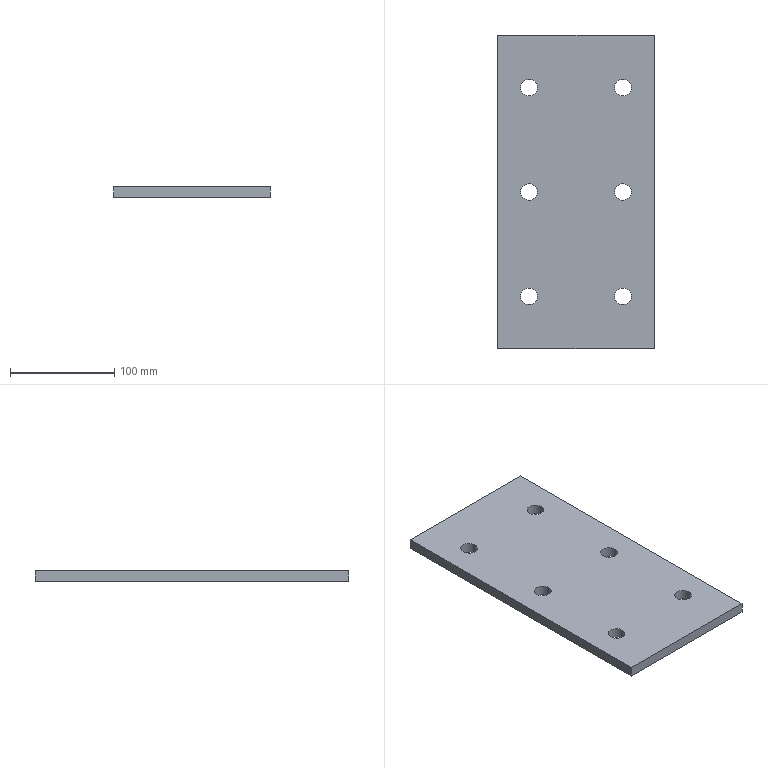Part | SolidWorks | features Extrusion 1 | 1 solid | 18 faces | box 150 x 300 x 10 mm | volume 437936 mm3 | cylinder 12 | plane 6 | commonest cylinder face diameters 16 x12
STEP:
#1=CARTESIAN_POINT('',(37.,100.,10.));
#2=VERTEX_POINT('',#1);
#3=CARTESIAN_POINT('',(53.,100.,10.));
#4=VERTEX_POINT('',#3);
#5=CARTESIAN_POINT('',(45.,100.,10.));
#6=DIRECTION('',(0.,0.,1.));
#7=DIRECTION('',(-1.,0.,0.));
#8=AXIS2_PLACEMENT_3D('',#5,#6,#7);
#9=CIRCLE('',#8,8.);
#10=EDGE_CURVE('',#2,#4,#9,.T.);
#11=ORIENTED_EDGE('',*,*,#10,.T.);
#12=CARTESIAN_POINT('',(53.,100.,0.));
#13=VERTEX_POINT('',#12);
#14=CARTESIAN_POINT('',(53.,100.,10.));
#15=DIRECTION('',(0.,0.,-1.));
#16=VECTOR('',#15,1000.);
#17=LINE('',#14,#16);
#18=EDGE_CURVE('',#4,#13,#17,.T.);
#19=ORIENTED_EDGE('',*,*,#18,.T.);
#20=CARTESIAN_POINT('',(37.,100.,0.));
#21=VERTEX_POINT('',#20);
#22=CARTESIAN_POINT('',(45.,100.,0.));
#23=DIRECTION('',(0.,0.,1.));
#24=DIRECTION('',(-1.,0.,0.));
#25=AXIS2_PLACEMENT_3D('',#22,#23,#24);
#26=CIRCLE('',#25,8.);
#27=EDGE_CURVE('',#21,#13,#26,.T.);
#28=ORIENTED_EDGE('',*,*,#27,.F.);
#29=CARTESIAN_POINT('',(37.,100.,10.));
#30=DIRECTION('',(0.,0.,-1.));
#31=VECTOR('',#30,1000.);
#32=LINE('',#29,#31);
#33=EDGE_CURVE('',#2,#21,#32,.T.);
#34=ORIENTED_EDGE('',*,*,#33,.F.);
#35=EDGE_LOOP('',(#11,#19,#28,#34));
#36=FACE_OUTER_BOUND('',#35,.T.);
#37=CARTESIAN_POINT('',(45.,100.,10.));
#38=DIRECTION('',(0.,0.,-1.));
#39=DIRECTION('',(-1.,0.,0.));
#40=AXIS2_PLACEMENT_3D('',#37,#38,#39);
#41=CYLINDRICAL_SURFACE('',#40,8.);
#42=ADVANCED_FACE('',(#36),#41,.F.);
#43=CARTESIAN_POINT('',(37.,0.,10.));
#44=VERTEX_POINT('',#43);
#45=CARTESIAN_POINT('',(53.,0.,10.));
#46=VERTEX_POINT('',#45);
#47=CARTESIAN_POINT('',(45.,0.,10.));
#48=DIRECTION('',(0.,0.,1.));
#49=DIRECTION('',(-1.,0.,0.));
#50=AXIS2_PLACEMENT_3D('',#47,#48,#49);
#51=CIRCLE('',#50,8.);
#52=EDGE_CURVE('',#44,#46,#51,.T.);
#53=ORIENTED_EDGE('',*,*,#52,.T.);
#54=CARTESIAN_POINT('',(53.,0.,0.));
#55=VERTEX_POINT('',#54);
#56=CARTESIAN_POINT('',(53.,0.,10.));
#57=DIRECTION('',(0.,0.,-1.));
#58=VECTOR('',#57,1000.);
#59=LINE('',#56,#58);
#60=EDGE_CURVE('',#46,#55,#59,.T.);
#61=ORIENTED_EDGE('',*,*,#60,.T.);
#62=CARTESIAN_POINT('',(37.,0.,0.));
#63=VERTEX_POINT('',#62);
#64=CARTESIAN_POINT('',(45.,0.,0.));
#65=DIRECTION('',(0.,0.,1.));
#66=DIRECTION('',(-1.,0.,0.));
#67=AXIS2_PLACEMENT_3D('',#64,#65,#66);
#68=CIRCLE('',#67,8.);
#69=EDGE_CURVE('',#63,#55,#68,.T.);
#70=ORIENTED_EDGE('',*,*,#69,.F.);
#71=CARTESIAN_POINT('',(37.,0.,10.));
#72=DIRECTION('',(0.,0.,-1.));
#73=VECTOR('',#72,1000.);
#74=LINE('',#71,#73);
#75=EDGE_CURVE('',#44,#63,#74,.T.);
#76=ORIENTED_EDGE('',*,*,#75,.F.);
#77=EDGE_LOOP('',(#53,#61,#70,#76));
#78=FACE_OUTER_BOUND('',#77,.T.);
#79=CARTESIAN_POINT('',(45.,0.,10.));
#80=DIRECTION('',(0.,0.,-1.));
#81=DIRECTION('',(-1.,0.,0.));
#82=AXIS2_PLACEMENT_3D('',#79,#80,#81);
#83=CYLINDRICAL_SURFACE('',#82,8.);
#84=ADVANCED_FACE('',(#78),#83,.F.);
#85=CARTESIAN_POINT('',(37.,-100.,10.));
#86=VERTEX_POINT('',#85);
#87=CARTESIAN_POINT('',(53.,-100.,10.));
#88=VERTEX_POINT('',#87);
#89=CARTESIAN_POINT('',(45.,-100.,10.));
#90=DIRECTION('',(0.,0.,1.));
#91=DIRECTION('',(-1.,0.,0.));
#92=AXIS2_PLACEMENT_3D('',#89,#90,#91);
#93=CIRCLE('',#92,8.);
#94=EDGE_CURVE('',#86,#88,#93,.T.);
#95=ORIENTED_EDGE('',*,*,#94,.T.);
#96=CARTESIAN_POINT('',(53.,-100.,0.));
#97=VERTEX_POINT('',#96);
#98=CARTESIAN_POINT('',(53.,-100.,10.));
#99=DIRECTION('',(0.,0.,-1.));
#100=VECTOR('',#99,1000.);
#101=LINE('',#98,#100);
#102=EDGE_CURVE('',#88,#97,#101,.T.);
#103=ORIENTED_EDGE('',*,*,#102,.T.);
#104=CARTESIAN_POINT('',(37.,-100.,0.));
#105=VERTEX_POINT('',#104);
#106=CARTESIAN_POINT('',(45.,-100.,0.));
#107=DIRECTION('',(0.,0.,1.));
#108=DIRECTION('',(-1.,0.,0.));
#109=AXIS2_PLACEMENT_3D('',#106,#107,#108);
#110=CIRCLE('',#109,8.);
#111=EDGE_CURVE('',#105,#97,#110,.T.);
#112=ORIENTED_EDGE('',*,*,#111,.F.);
#113=CARTESIAN_POINT('',(37.,-100.,10.));
#114=DIRECTION('',(0.,0.,-1.));
#115=VECTOR('',#114,1000.);
#116=LINE('',#113,#115);
#117=EDGE_CURVE('',#86,#105,#116,.T.);
#118=ORIENTED_EDGE('',*,*,#117,.F.);
#119=EDGE_LOOP('',(#95,#103,#112,#118));
#120=FACE_OUTER_BOUND('',#119,.T.);
#121=CARTESIAN_POINT('',(45.,-100.,10.));
#122=DIRECTION('',(0.,0.,-1.));
#123=DIRECTION('',(-1.,0.,0.));
#124=AXIS2_PLACEMENT_3D('',#121,#122,#123);
#125=CYLINDRICAL_SURFACE('',#124,8.);
#126=ADVANCED_FACE('',(#120),#125,.F.);
#127=CARTESIAN_POINT('',(-53.,-100.,10.));
#128=VERTEX_POINT('',#127);
#129=CARTESIAN_POINT('',(-37.,-100.,10.));
#130=VERTEX_POINT('',#129);
#131=CARTESIAN_POINT('',(-45.,-100.,10.));
#132=DIRECTION('',(0.,0.,1.));
#133=DIRECTION('',(1.,0.,0.));
#134=AXIS2_PLACEMENT_3D('',#131,#132,#133);
#135=CIRCLE('',#134,8.);
#136=EDGE_CURVE('',#128,#130,#135,.T.);
#137=ORIENTED_EDGE('',*,*,#136,.T.);
#138=CARTESIAN_POINT('',(-37.,-100.,0.));
#139=VERTEX_POINT('',#138);
#140=CARTESIAN_POINT('',(-37.,-100.,10.));
#141=DIRECTION('',(0.,0.,-1.));
#142=VECTOR('',#141,1000.);
#143=LINE('',#140,#142);
#144=EDGE_CURVE('',#130,#139,#143,.T.);
#145=ORIENTED_EDGE('',*,*,#144,.T.);
#146=CARTESIAN_POINT('',(-53.,-100.,0.));
#147=VERTEX_POINT('',#146);
#148=CARTESIAN_POINT('',(-45.,-100.,0.));
#149=DIRECTION('',(0.,0.,1.));
#150=DIRECTION('',(1.,0.,0.));
#151=AXIS2_PLACEMENT_3D('',#148,#149,#150);
#152=CIRCLE('',#151,8.);
#153=EDGE_CURVE('',#147,#139,#152,.T.);
#154=ORIENTED_EDGE('',*,*,#153,.F.);
#155=CARTESIAN_POINT('',(-53.,-100.,10.));
#156=DIRECTION('',(0.,0.,-1.));
#157=VECTOR('',#156,1000.);
#158=LINE('',#155,#157);
#159=EDGE_CURVE('',#128,#147,#158,.T.);
#160=ORIENTED_EDGE('',*,*,#159,.F.);
#161=EDGE_LOOP('',(#137,#145,#154,#160));
#162=FACE_OUTER_BOUND('',#161,.T.);
#163=CARTESIAN_POINT('',(-45.,-100.,10.));
#164=DIRECTION('',(0.,0.,-1.));
#165=DIRECTION('',(-1.,0.,0.));
#166=AXIS2_PLACEMENT_3D('',#163,#164,#165);
#167=CYLINDRICAL_SURFACE('',#166,8.);
#168=ADVANCED_FACE('',(#162),#167,.F.);
#169=CARTESIAN_POINT('',(-53.,0.,10.));
#170=VERTEX_POINT('',#169);
#171=CARTESIAN_POINT('',(-37.,0.,10.));
#172=VERTEX_POINT('',#171);
#173=CARTESIAN_POINT('',(-45.,0.,10.));
#174=DIRECTION('',(0.,0.,1.));
#175=DIRECTION('',(1.,0.,0.));
#176=AXIS2_PLACEMENT_3D('',#173,#174,#175);
#177=CIRCLE('',#176,8.);
#178=EDGE_CURVE('',#170,#172,#177,.T.);
#179=ORIENTED_EDGE('',*,*,#178,.T.);
#180=CARTESIAN_POINT('',(-37.,0.,0.));
#181=VERTEX_POINT('',#180);
#182=CARTESIAN_POINT('',(-37.,0.,10.));
#183=DIRECTION('',(0.,0.,-1.));
#184=VECTOR('',#183,1000.);
#185=LINE('',#182,#184);
#186=EDGE_CURVE('',#172,#181,#185,.T.);
#187=ORIENTED_EDGE('',*,*,#186,.T.);
#188=CARTESIAN_POINT('',(-53.,0.,0.));
#189=VERTEX_POINT('',#188);
#190=CARTESIAN_POINT('',(-45.,0.,0.));
#191=DIRECTION('',(0.,0.,1.));
#192=DIRECTION('',(1.,0.,0.));
#193=AXIS2_PLACEMENT_3D('',#190,#191,#192);
#194=CIRCLE('',#193,8.);
#195=EDGE_CURVE('',#189,#181,#194,.T.);
#196=ORIENTED_EDGE('',*,*,#195,.F.);
#197=CARTESIAN_POINT('',(-53.,0.,10.));
#198=DIRECTION('',(0.,0.,-1.));
#199=VECTOR('',#198,1000.);
#200=LINE('',#197,#199);
#201=EDGE_CURVE('',#170,#189,#200,.T.);
#202=ORIENTED_EDGE('',*,*,#201,.F.);
#203=EDGE_LOOP('',(#179,#187,#196,#202));
#204=FACE_OUTER_BOUND('',#203,.T.);
#205=CARTESIAN_POINT('',(-45.,0.,10.));
#206=DIRECTION('',(0.,0.,-1.));
#207=DIRECTION('',(-1.,0.,0.));
#208=AXIS2_PLACEMENT_3D('',#205,#206,#207);
#209=CYLINDRICAL_SURFACE('',#208,8.);
#210=ADVANCED_FACE('',(#204),#209,.F.);
#211=CARTESIAN_POINT('',(-53.,100.,10.));
#212=VERTEX_POINT('',#211);
#213=CARTESIAN_POINT('',(-37.,100.,10.));
#214=VERTEX_POINT('',#213);
#215=CARTESIAN_POINT('',(-45.,100.,10.));
#216=DIRECTION('',(0.,0.,1.));
#217=DIRECTION('',(1.,0.,0.));
#218=AXIS2_PLACEMENT_3D('',#215,#216,#217);
#219=CIRCLE('',#218,8.);
#220=EDGE_CURVE('',#212,#214,#219,.T.);
#221=ORIENTED_EDGE('',*,*,#220,.T.);
#222=CARTESIAN_POINT('',(-37.,100.,0.));
#223=VERTEX_POINT('',#222);
#224=CARTESIAN_POINT('',(-37.,100.,10.));
#225=DIRECTION('',(0.,0.,-1.));
#226=VECTOR('',#225,1000.);
#227=LINE('',#224,#226);
#228=EDGE_CURVE('',#214,#223,#227,.T.);
#229=ORIENTED_EDGE('',*,*,#228,.T.);
#230=CARTESIAN_POINT('',(-53.,100.,0.));
#231=VERTEX_POINT('',#230);
#232=CARTESIAN_POINT('',(-45.,100.,0.));
#233=DIRECTION('',(0.,0.,1.));
#234=DIRECTION('',(1.,0.,0.));
#235=AXIS2_PLACEMENT_3D('',#232,#233,#234);
#236=CIRCLE('',#235,8.);
#237=EDGE_CURVE('',#231,#223,#236,.T.);
#238=ORIENTED_EDGE('',*,*,#237,.F.);
#239=CARTESIAN_POINT('',(-53.,100.,10.));
#240=DIRECTION('',(0.,0.,-1.));
#241=VECTOR('',#240,1000.);
#242=LINE('',#239,#241);
#243=EDGE_CURVE('',#212,#231,#242,.T.);
#244=ORIENTED_EDGE('',*,*,#243,.F.);
#245=EDGE_LOOP('',(#221,#229,#238,#244));
#246=FACE_OUTER_BOUND('',#245,.T.);
#247=CARTESIAN_POINT('',(-45.,100.,10.));
#248=DIRECTION('',(0.,0.,-1.));
#249=DIRECTION('',(-1.,0.,0.));
#250=AXIS2_PLACEMENT_3D('',#247,#248,#249);
#251=CYLINDRICAL_SURFACE('',#250,8.);
#252=ADVANCED_FACE('',(#246),#251,.F.);
#253=CARTESIAN_POINT('',(-75.,150.,10.));
#254=VERTEX_POINT('',#253);
#255=CARTESIAN_POINT('',(-75.,-150.,10.));
#256=VERTEX_POINT('',#255);
#257=CARTESIAN_POINT('',(-75.,150.,10.));
#258=DIRECTION('',(0.,-1.,0.));
#259=VECTOR('',#258,1000.);
#260=LINE('',#257,#259);
#261=EDGE_CURVE('',#254,#256,#260,.T.);
#262=ORIENTED_EDGE('',*,*,#261,.T.);
#263=CARTESIAN_POINT('',(75.,-150.,10.));
#264=VERTEX_POINT('',#263);
#265=CARTESIAN_POINT('',(75.,-150.,10.));
#266=DIRECTION('',(1.,0.,0.));
#267=VECTOR('',#266,1000.);
#268=LINE('',#265,#267);
#269=EDGE_CURVE('',#256,#264,#268,.T.);
#270=ORIENTED_EDGE('',*,*,#269,.T.);
#271=CARTESIAN_POINT('',(75.,150.,10.));
#272=VERTEX_POINT('',#271);
#273=CARTESIAN_POINT('',(75.,150.,10.));
#274=DIRECTION('',(0.,1.,0.));
#275=VECTOR('',#274,1000.);
#276=LINE('',#273,#275);
#277=EDGE_CURVE('',#264,#272,#276,.T.);
#278=ORIENTED_EDGE('',*,*,#277,.T.);
#279=CARTESIAN_POINT('',(75.,150.,10.));
#280=DIRECTION('',(-1.,0.,0.));
#281=VECTOR('',#280,1000.);
#282=LINE('',#279,#281);
#283=EDGE_CURVE('',#272,#254,#282,.T.);
#284=ORIENTED_EDGE('',*,*,#283,.T.);
#285=EDGE_LOOP('',(#262,#270,#278,#284));
#286=FACE_OUTER_BOUND('',#285,.T.);
#287=ORIENTED_EDGE('',*,*,#220,.F.);
#288=CARTESIAN_POINT('',(-45.,100.,10.));
#289=DIRECTION('',(0.,0.,1.));
#290=DIRECTION('',(1.,0.,0.));
#291=AXIS2_PLACEMENT_3D('',#288,#289,#290);
#292=CIRCLE('',#291,8.);
#293=EDGE_CURVE('',#214,#212,#292,.T.);
#294=ORIENTED_EDGE('',*,*,#293,.F.);
#295=EDGE_LOOP('',(#287,#294));
#296=FACE_BOUND('',#295,.T.);
#297=ORIENTED_EDGE('',*,*,#178,.F.);
#298=CARTESIAN_POINT('',(-45.,0.,10.));
#299=DIRECTION('',(0.,0.,1.));
#300=DIRECTION('',(1.,0.,0.));
#301=AXIS2_PLACEMENT_3D('',#298,#299,#300);
#302=CIRCLE('',#301,8.);
#303=EDGE_CURVE('',#172,#170,#302,.T.);
#304=ORIENTED_EDGE('',*,*,#303,.F.);
#305=EDGE_LOOP('',(#297,#304));
#306=FACE_BOUND('',#305,.T.);
#307=ORIENTED_EDGE('',*,*,#136,.F.);
#308=CARTESIAN_POINT('',(-45.,-100.,10.));
#309=DIRECTION('',(0.,0.,1.));
#310=DIRECTION('',(1.,0.,0.));
#311=AXIS2_PLACEMENT_3D('',#308,#309,#310);
#312=CIRCLE('',#311,8.);
#313=EDGE_CURVE('',#130,#128,#312,.T.);
#314=ORIENTED_EDGE('',*,*,#313,.F.);
#315=EDGE_LOOP('',(#307,#314));
#316=FACE_BOUND('',#315,.T.);
#317=ORIENTED_EDGE('',*,*,#94,.F.);
#318=CARTESIAN_POINT('',(45.,-100.,10.));
#319=DIRECTION('',(0.,0.,1.));
#320=DIRECTION('',(-1.,0.,0.));
#321=AXIS2_PLACEMENT_3D('',#318,#319,#320);
#322=CIRCLE('',#321,8.);
#323=EDGE_CURVE('',#88,#86,#322,.T.);
#324=ORIENTED_EDGE('',*,*,#323,.F.);
#325=EDGE_LOOP('',(#317,#324));
#326=FACE_BOUND('',#325,.T.);
#327=ORIENTED_EDGE('',*,*,#52,.F.);
#328=CARTESIAN_POINT('',(45.,0.,10.));
#329=DIRECTION('',(0.,0.,1.));
#330=DIRECTION('',(-1.,0.,0.));
#331=AXIS2_PLACEMENT_3D('',#328,#329,#330);
#332=CIRCLE('',#331,8.);
#333=EDGE_CURVE('',#46,#44,#332,.T.);
#334=ORIENTED_EDGE('',*,*,#333,.F.);
#335=EDGE_LOOP('',(#327,#334));
#336=FACE_BOUND('',#335,.T.);
#337=ORIENTED_EDGE('',*,*,#10,.F.);
#338=CARTESIAN_POINT('',(45.,100.,10.));
#339=DIRECTION('',(0.,0.,1.));
#340=DIRECTION('',(-1.,0.,0.));
#341=AXIS2_PLACEMENT_3D('',#338,#339,#340);
#342=CIRCLE('',#341,8.);
#343=EDGE_CURVE('',#4,#2,#342,.T.);
#344=ORIENTED_EDGE('',*,*,#343,.F.);
#345=EDGE_LOOP('',(#337,#344));
#346=FACE_BOUND('',#345,.T.);
#347=CARTESIAN_POINT('',(0.,0.,10.));
#348=DIRECTION('',(0.,0.,-1.));
#349=DIRECTION('',(-1.,0.,0.));
#350=AXIS2_PLACEMENT_3D('',#347,#348,#349);
#351=PLANE('',#350);
#352=ADVANCED_FACE('',(#286,#296,#306,#316,#326,#336,#346),#351,.F.);
#353=ORIENTED_EDGE('',*,*,#69,.T.);
#354=CARTESIAN_POINT('',(45.,0.,0.));
#355=DIRECTION('',(0.,0.,1.));
#356=DIRECTION('',(-1.,0.,0.));
#357=AXIS2_PLACEMENT_3D('',#354,#355,#356);
#358=CIRCLE('',#357,8.);
#359=EDGE_CURVE('',#55,#63,#358,.T.);
#360=ORIENTED_EDGE('',*,*,#359,.T.);
#361=EDGE_LOOP('',(#353,#360));
#362=FACE_BOUND('',#361,.T.);
#363=ORIENTED_EDGE('',*,*,#153,.T.);
#364=CARTESIAN_POINT('',(-45.,-100.,0.));
#365=DIRECTION('',(0.,0.,1.));
#366=DIRECTION('',(1.,0.,0.));
#367=AXIS2_PLACEMENT_3D('',#364,#365,#366);
#368=CIRCLE('',#367,8.);
#369=EDGE_CURVE('',#139,#147,#368,.T.);
#370=ORIENTED_EDGE('',*,*,#369,.T.);
#371=EDGE_LOOP('',(#363,#370));
#372=FACE_BOUND('',#371,.T.);
#373=ORIENTED_EDGE('',*,*,#237,.T.);
#374=CARTESIAN_POINT('',(-45.,100.,0.));
#375=DIRECTION('',(0.,0.,1.));
#376=DIRECTION('',(1.,0.,0.));
#377=AXIS2_PLACEMENT_3D('',#374,#375,#376);
#378=CIRCLE('',#377,8.);
#379=EDGE_CURVE('',#223,#231,#378,.T.);
#380=ORIENTED_EDGE('',*,*,#379,.T.);
#381=EDGE_LOOP('',(#373,#380));
#382=FACE_BOUND('',#381,.T.);
#383=CARTESIAN_POINT('',(-75.,150.,0.));
#384=VERTEX_POINT('',#383);
#385=CARTESIAN_POINT('',(-75.,-150.,0.));
#386=VERTEX_POINT('',#385);
#387=CARTESIAN_POINT('',(-75.,150.,0.));
#388=DIRECTION('',(0.,-1.,0.));
#389=VECTOR('',#388,1000.);
#390=LINE('',#387,#389);
#391=EDGE_CURVE('',#384,#386,#390,.T.);
#392=ORIENTED_EDGE('',*,*,#391,.F.);
#393=CARTESIAN_POINT('',(75.,150.,0.));
#394=VERTEX_POINT('',#393);
#395=CARTESIAN_POINT('',(75.,150.,0.));
#396=DIRECTION('',(-1.,0.,0.));
#397=VECTOR('',#396,1000.);
#398=LINE('',#395,#397);
#399=EDGE_CURVE('',#394,#384,#398,.T.);
#400=ORIENTED_EDGE('',*,*,#399,.F.);
#401=CARTESIAN_POINT('',(75.,-150.,0.));
#402=VERTEX_POINT('',#401);
#403=CARTESIAN_POINT('',(75.,150.,0.));
#404=DIRECTION('',(0.,1.,0.));
#405=VECTOR('',#404,1000.);
#406=LINE('',#403,#405);
#407=EDGE_CURVE('',#402,#394,#406,.T.);
#408=ORIENTED_EDGE('',*,*,#407,.F.);
#409=CARTESIAN_POINT('',(75.,-150.,0.));
#410=DIRECTION('',(1.,0.,0.));
#411=VECTOR('',#410,1000.);
#412=LINE('',#409,#411);
#413=EDGE_CURVE('',#386,#402,#412,.T.);
#414=ORIENTED_EDGE('',*,*,#413,.F.);
#415=EDGE_LOOP('',(#392,#400,#408,#414));
#416=FACE_OUTER_BOUND('',#415,.T.);
#417=ORIENTED_EDGE('',*,*,#195,.T.);
#418=CARTESIAN_POINT('',(-45.,0.,0.));
#419=DIRECTION('',(0.,0.,1.));
#420=DIRECTION('',(1.,0.,0.));
#421=AXIS2_PLACEMENT_3D('',#418,#419,#420);
#422=CIRCLE('',#421,8.);
#423=EDGE_CURVE('',#181,#189,#422,.T.);
#424=ORIENTED_EDGE('',*,*,#423,.T.);
#425=EDGE_LOOP('',(#417,#424));
#426=FACE_BOUND('',#425,.T.);
#427=ORIENTED_EDGE('',*,*,#111,.T.);
#428=CARTESIAN_POINT('',(45.,-100.,0.));
#429=DIRECTION('',(0.,0.,1.));
#430=DIRECTION('',(-1.,0.,0.));
#431=AXIS2_PLACEMENT_3D('',#428,#429,#430);
#432=CIRCLE('',#431,8.);
#433=EDGE_CURVE('',#97,#105,#432,.T.);
#434=ORIENTED_EDGE('',*,*,#433,.T.);
#435=EDGE_LOOP('',(#427,#434));
#436=FACE_BOUND('',#435,.T.);
#437=ORIENTED_EDGE('',*,*,#27,.T.);
#438=CARTESIAN_POINT('',(45.,100.,0.));
#439=DIRECTION('',(0.,0.,1.));
#440=DIRECTION('',(-1.,0.,0.));
#441=AXIS2_PLACEMENT_3D('',#438,#439,#440);
#442=CIRCLE('',#441,8.);
#443=EDGE_CURVE('',#13,#21,#442,.T.);
#444=ORIENTED_EDGE('',*,*,#443,.T.);
#445=EDGE_LOOP('',(#437,#444));
#446=FACE_BOUND('',#445,.T.);
#447=CARTESIAN_POINT('',(0.,0.,0.));
#448=DIRECTION('',(0.,0.,-1.));
#449=DIRECTION('',(-1.,0.,0.));
#450=AXIS2_PLACEMENT_3D('',#447,#448,#449);
#451=PLANE('',#450);
#452=ADVANCED_FACE('',(#362,#372,#382,#416,#426,#436,#446),#451,.T.);
#453=ORIENTED_EDGE('',*,*,#391,.T.);
#454=CARTESIAN_POINT('',(-75.,-150.,10.));
#455=DIRECTION('',(0.,0.,-1.));
#456=VECTOR('',#455,1000.);
#457=LINE('',#454,#456);
#458=EDGE_CURVE('',#256,#386,#457,.T.);
#459=ORIENTED_EDGE('',*,*,#458,.F.);
#460=ORIENTED_EDGE('',*,*,#261,.F.);
#461=CARTESIAN_POINT('',(-75.,150.,10.));
#462=DIRECTION('',(0.,0.,-1.));
#463=VECTOR('',#462,1000.);
#464=LINE('',#461,#463);
#465=EDGE_CURVE('',#254,#384,#464,.T.);
#466=ORIENTED_EDGE('',*,*,#465,.T.);
#467=EDGE_LOOP('',(#453,#459,#460,#466));
#468=FACE_OUTER_BOUND('',#467,.T.);
#469=CARTESIAN_POINT('',(-75.,150.,10.));
#470=DIRECTION('',(1.,0.,0.));
#471=DIRECTION('',(0.,1.,0.));
#472=AXIS2_PLACEMENT_3D('',#469,#470,#471);
#473=PLANE('',#472);
#474=ADVANCED_FACE('',(#468),#473,.F.);
#475=ORIENTED_EDGE('',*,*,#413,.T.);
#476=CARTESIAN_POINT('',(75.,-150.,10.));
#477=DIRECTION('',(0.,0.,-1.));
#478=VECTOR('',#477,1000.);
#479=LINE('',#476,#478);
#480=EDGE_CURVE('',#264,#402,#479,.T.);
#481=ORIENTED_EDGE('',*,*,#480,.F.);
#482=ORIENTED_EDGE('',*,*,#269,.F.);
#483=ORIENTED_EDGE('',*,*,#458,.T.);
#484=EDGE_LOOP('',(#475,#481,#482,#483));
#485=FACE_OUTER_BOUND('',#484,.T.);
#486=CARTESIAN_POINT('',(75.,-150.,10.));
#487=DIRECTION('',(0.,1.,0.));
#488=DIRECTION('',(-1.,0.,0.));
#489=AXIS2_PLACEMENT_3D('',#486,#487,#488);
#490=PLANE('',#489);
#491=ADVANCED_FACE('',(#485),#490,.F.);
#492=ORIENTED_EDGE('',*,*,#407,.T.);
#493=CARTESIAN_POINT('',(75.,150.,10.));
#494=DIRECTION('',(0.,0.,-1.));
#495=VECTOR('',#494,1000.);
#496=LINE('',#493,#495);
#497=EDGE_CURVE('',#272,#394,#496,.T.);
#498=ORIENTED_EDGE('',*,*,#497,.F.);
#499=ORIENTED_EDGE('',*,*,#277,.F.);
#500=ORIENTED_EDGE('',*,*,#480,.T.);
#501=EDGE_LOOP('',(#492,#498,#499,#500));
#502=FACE_OUTER_BOUND('',#501,.T.);
#503=CARTESIAN_POINT('',(75.,150.,10.));
#504=DIRECTION('',(-1.,0.,0.));
#505=DIRECTION('',(0.,-1.,0.));
#506=AXIS2_PLACEMENT_3D('',#503,#504,#505);
#507=PLANE('',#506);
#508=ADVANCED_FACE('',(#502),#507,.F.);
#509=ORIENTED_EDGE('',*,*,#399,.T.);
#510=ORIENTED_EDGE('',*,*,#465,.F.);
#511=ORIENTED_EDGE('',*,*,#283,.F.);
#512=ORIENTED_EDGE('',*,*,#497,.T.);
#513=EDGE_LOOP('',(#509,#510,#511,#512));
#514=FACE_OUTER_BOUND('',#513,.T.);
#515=CARTESIAN_POINT('',(75.,150.,10.));
#516=DIRECTION('',(0.,-1.,0.));
#517=DIRECTION('',(1.,0.,0.));
#518=AXIS2_PLACEMENT_3D('',#515,#516,#517);
#519=PLANE('',#518);
#520=ADVANCED_FACE('',(#514),#519,.F.);
#521=ORIENTED_EDGE('',*,*,#228,.F.);
#522=ORIENTED_EDGE('',*,*,#293,.T.);
#523=ORIENTED_EDGE('',*,*,#243,.T.);
#524=ORIENTED_EDGE('',*,*,#379,.F.);
#525=EDGE_LOOP('',(#521,#522,#523,#524));
#526=FACE_OUTER_BOUND('',#525,.T.);
#527=CARTESIAN_POINT('',(-45.,100.,10.));
#528=DIRECTION('',(0.,0.,-1.));
#529=DIRECTION('',(-1.,0.,0.));
#530=AXIS2_PLACEMENT_3D('',#527,#528,#529);
#531=CYLINDRICAL_SURFACE('',#530,8.);
#532=ADVANCED_FACE('',(#526),#531,.F.);
#533=ORIENTED_EDGE('',*,*,#186,.F.);
#534=ORIENTED_EDGE('',*,*,#303,.T.);
#535=ORIENTED_EDGE('',*,*,#201,.T.);
#536=ORIENTED_EDGE('',*,*,#423,.F.);
#537=EDGE_LOOP('',(#533,#534,#535,#536));
#538=FACE_OUTER_BOUND('',#537,.T.);
#539=CARTESIAN_POINT('',(-45.,0.,10.));
#540=DIRECTION('',(0.,0.,-1.));
#541=DIRECTION('',(-1.,0.,0.));
#542=AXIS2_PLACEMENT_3D('',#539,#540,#541);
#543=CYLINDRICAL_SURFACE('',#542,8.);
#544=ADVANCED_FACE('',(#538),#543,.F.);
#545=ORIENTED_EDGE('',*,*,#144,.F.);
#546=ORIENTED_EDGE('',*,*,#313,.T.);
#547=ORIENTED_EDGE('',*,*,#159,.T.);
#548=ORIENTED_EDGE('',*,*,#369,.F.);
#549=EDGE_LOOP('',(#545,#546,#547,#548));
#550=FACE_OUTER_BOUND('',#549,.T.);
#551=CARTESIAN_POINT('',(-45.,-100.,10.));
#552=DIRECTION('',(0.,0.,-1.));
#553=DIRECTION('',(-1.,0.,0.));
#554=AXIS2_PLACEMENT_3D('',#551,#552,#553);
#555=CYLINDRICAL_SURFACE('',#554,8.);
#556=ADVANCED_FACE('',(#550),#555,.F.);
#557=ORIENTED_EDGE('',*,*,#102,.F.);
#558=ORIENTED_EDGE('',*,*,#323,.T.);
#559=ORIENTED_EDGE('',*,*,#117,.T.);
#560=ORIENTED_EDGE('',*,*,#433,.F.);
#561=EDGE_LOOP('',(#557,#558,#559,#560));
#562=FACE_OUTER_BOUND('',#561,.T.);
#563=CARTESIAN_POINT('',(45.,-100.,10.));
#564=DIRECTION('',(0.,0.,-1.));
#565=DIRECTION('',(-1.,0.,0.));
#566=AXIS2_PLACEMENT_3D('',#563,#564,#565);
#567=CYLINDRICAL_SURFACE('',#566,8.);
#568=ADVANCED_FACE('',(#562),#567,.F.);
#569=ORIENTED_EDGE('',*,*,#60,.F.);
#570=ORIENTED_EDGE('',*,*,#333,.T.);
#571=ORIENTED_EDGE('',*,*,#75,.T.);
#572=ORIENTED_EDGE('',*,*,#359,.F.);
#573=EDGE_LOOP('',(#569,#570,#571,#572));
#574=FACE_OUTER_BOUND('',#573,.T.);
#575=CARTESIAN_POINT('',(45.,0.,10.));
#576=DIRECTION('',(0.,0.,-1.));
#577=DIRECTION('',(-1.,0.,0.));
#578=AXIS2_PLACEMENT_3D('',#575,#576,#577);
#579=CYLINDRICAL_SURFACE('',#578,8.);
#580=ADVANCED_FACE('',(#574),#579,.F.);
#581=ORIENTED_EDGE('',*,*,#18,.F.);
#582=ORIENTED_EDGE('',*,*,#343,.T.);
#583=ORIENTED_EDGE('',*,*,#33,.T.);
#584=ORIENTED_EDGE('',*,*,#443,.F.);
#585=EDGE_LOOP('',(#581,#582,#583,#584));
#586=FACE_OUTER_BOUND('',#585,.T.);
#587=CARTESIAN_POINT('',(45.,100.,10.));
#588=DIRECTION('',(0.,0.,-1.));
#589=DIRECTION('',(-1.,0.,0.));
#590=AXIS2_PLACEMENT_3D('',#587,#588,#589);
#591=CYLINDRICAL_SURFACE('',#590,8.);
#592=ADVANCED_FACE('',(#586),#591,.F.);
#593=CLOSED_SHELL('',(#42,#84,#126,#168,#210,#252,#352,#452,#474,#491,#508,#520,#532,#544,#556,#568,#580,#592));
#594=MANIFOLD_SOLID_BREP('',#593);
#595=CARTESIAN_POINT('',(0.,0.,0.));
#596=DIRECTION('',(0.,0.,1.));
#597=DIRECTION('',(1.,0.,0.));
#598=AXIS2_PLACEMENT_3D('',#595,#596,#597);
#599=(LENGTH_UNIT()NAMED_UNIT(*)SI_UNIT(.MILLI.,.METRE.));
#600=UNCERTAINTY_MEASURE_WITH_UNIT(LENGTH_MEASURE(0.00001),#599,'','');
#601=(NAMED_UNIT(*)PLANE_ANGLE_UNIT()SI_UNIT($,.RADIAN.));
#602=(NAMED_UNIT(*)SI_UNIT($,.STERADIAN.)SOLID_ANGLE_UNIT());
#603=(GEOMETRIC_REPRESENTATION_CONTEXT(3)GLOBAL_UNCERTAINTY_ASSIGNED_CONTEXT((#600))GLOBAL_UNIT_ASSIGNED_CONTEXT((#599,#601,#602))REPRESENTATION_CONTEXT('',''));
#604=ADVANCED_BREP_SHAPE_REPRESENTATION('',(#594,#598),#603);